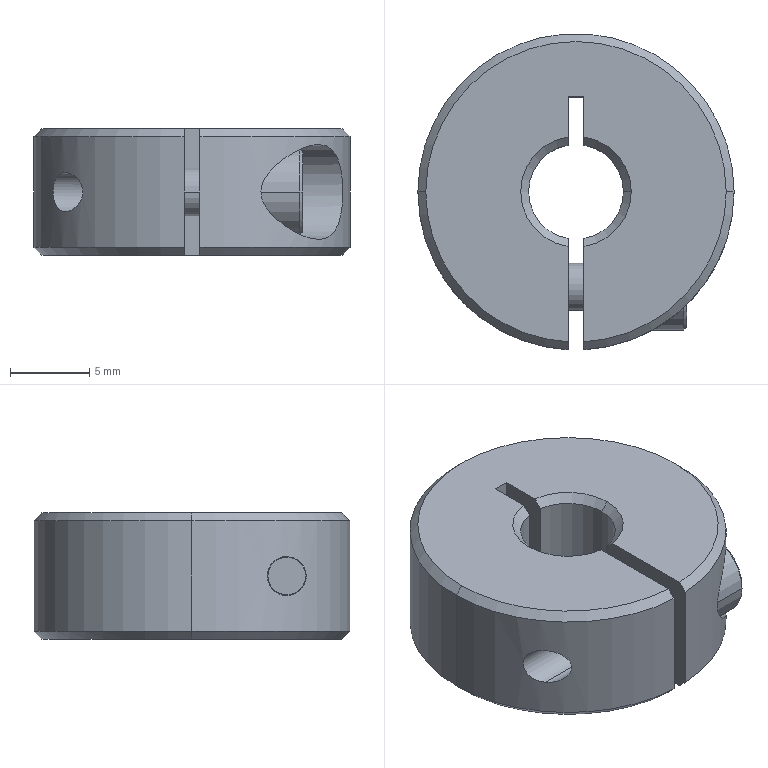Part | SolidWorks | features BaseBody 2 | 2 solids | 50 faces | box 20 x 19.987 x 8 mm | volume 2133 mm3 | plane 18 | cylinder 16 | cone 16 | commonest cylinder face diameters 6 x5 20 x3 2.459 x2 3 x2 3.4 x2 5.5 x2